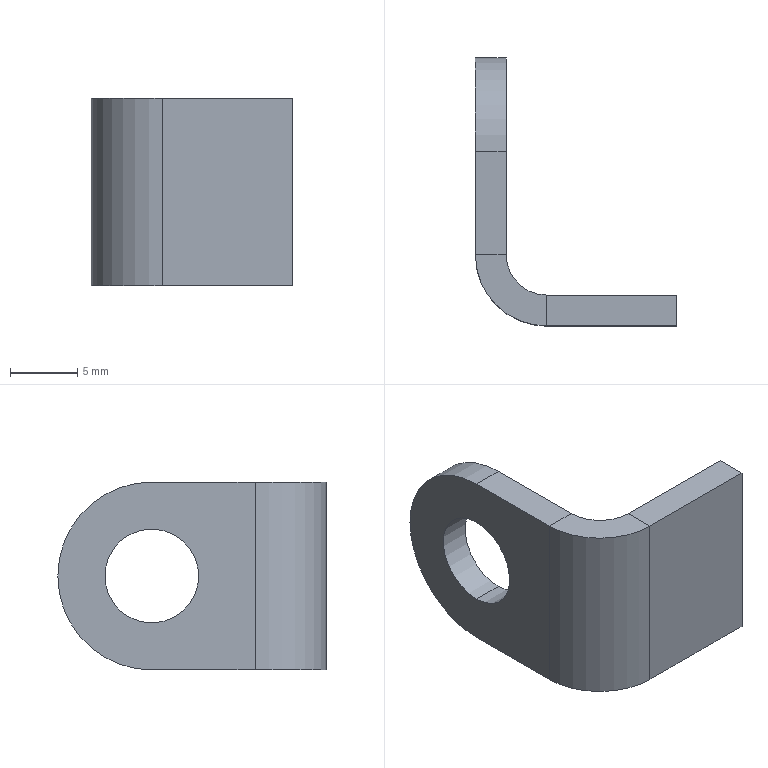Part | SolidWorks | features Fillet 1, FlatPattern 1, ICE 1, SMBaseFlange 1, SheetMetal 1 | 1 solid | 17 faces | box 15 x 20 x 14 mm | volume 858.7 mm3 | plane 11 | cylinder 6 | commonest cylinder face diameters 7 x2 14 x2 6 x1 10.6 x1
STEP:
#1=CARTESIAN_POINT('',(0.,13.,3.5));
#2=VERTEX_POINT('',#1);
#3=CARTESIAN_POINT('',(0.,13.,-3.5));
#4=VERTEX_POINT('',#3);
#5=CARTESIAN_POINT('',(0.,13.,0.));
#6=DIRECTION('',(1.,0.,0.));
#7=DIRECTION('',(0.,0.,-1.));
#8=AXIS2_PLACEMENT_3D('',#5,#6,#7);
#9=CIRCLE('',#8,3.5);
#10=EDGE_CURVE('',#2,#4,#9,.T.);
#11=ORIENTED_EDGE('',*,*,#10,.F.);
#12=CARTESIAN_POINT('',(2.3,13.,3.5));
#13=VERTEX_POINT('',#12);
#14=CARTESIAN_POINT('',(0.,13.,3.5));
#15=DIRECTION('',(1.,0.,0.));
#16=VECTOR('',#15,1000.);
#17=LINE('',#14,#16);
#18=EDGE_CURVE('',#2,#13,#17,.T.);
#19=ORIENTED_EDGE('',*,*,#18,.T.);
#20=CARTESIAN_POINT('',(2.3,13.,-3.5));
#21=VERTEX_POINT('',#20);
#22=CARTESIAN_POINT('',(2.3,13.,0.));
#23=DIRECTION('',(1.,0.,0.));
#24=DIRECTION('',(0.,0.,-1.));
#25=AXIS2_PLACEMENT_3D('',#22,#23,#24);
#26=CIRCLE('',#25,3.5);
#27=EDGE_CURVE('',#13,#21,#26,.T.);
#28=ORIENTED_EDGE('',*,*,#27,.T.);
#29=CARTESIAN_POINT('',(0.,13.,-3.5));
#30=DIRECTION('',(1.,0.,0.));
#31=VECTOR('',#30,1000.);
#32=LINE('',#29,#31);
#33=EDGE_CURVE('',#4,#21,#32,.T.);
#34=ORIENTED_EDGE('',*,*,#33,.F.);
#35=EDGE_LOOP('',(#11,#19,#28,#34));
#36=FACE_OUTER_BOUND('',#35,.T.);
#37=CARTESIAN_POINT('',(0.,13.,0.));
#38=DIRECTION('',(1.,0.,0.));
#39=DIRECTION('',(0.,0.,-1.));
#40=AXIS2_PLACEMENT_3D('',#37,#38,#39);
#41=CYLINDRICAL_SURFACE('',#40,3.5);
#42=ADVANCED_FACE('',(#36),#41,.F.);
#43=CARTESIAN_POINT('',(0.,5.3,7.));
#44=VERTEX_POINT('',#43);
#45=CARTESIAN_POINT('',(2.3,5.3,7.));
#46=VERTEX_POINT('',#45);
#47=CARTESIAN_POINT('',(0.,5.3,7.));
#48=DIRECTION('',(1.,0.,0.));
#49=VECTOR('',#48,1000.);
#50=LINE('',#47,#49);
#51=EDGE_CURVE('',#44,#46,#50,.T.);
#52=ORIENTED_EDGE('',*,*,#51,.F.);
#53=CARTESIAN_POINT('',(5.3,0.,7.));
#54=VERTEX_POINT('',#53);
#55=CARTESIAN_POINT('',(5.3,5.3,7.));
#56=DIRECTION('',(0.,0.,-1.));
#57=DIRECTION('',(1.,0.,0.));
#58=AXIS2_PLACEMENT_3D('',#55,#56,#57);
#59=CIRCLE('',#58,5.3);
#60=EDGE_CURVE('',#54,#44,#59,.T.);
#61=ORIENTED_EDGE('',*,*,#60,.F.);
#62=CARTESIAN_POINT('',(5.3,2.3,7.));
#63=VERTEX_POINT('',#62);
#64=CARTESIAN_POINT('',(5.3,2.3,7.));
#65=DIRECTION('',(0.,-1.,0.));
#66=VECTOR('',#65,1000.);
#67=LINE('',#64,#66);
#68=EDGE_CURVE('',#63,#54,#67,.T.);
#69=ORIENTED_EDGE('',*,*,#68,.F.);
#70=CARTESIAN_POINT('',(5.3,5.3,7.));
#71=DIRECTION('',(0.,0.,-1.));
#72=DIRECTION('',(1.,0.,0.));
#73=AXIS2_PLACEMENT_3D('',#70,#71,#72);
#74=CIRCLE('',#73,3.);
#75=EDGE_CURVE('',#63,#46,#74,.T.);
#76=ORIENTED_EDGE('',*,*,#75,.T.);
#77=EDGE_LOOP('',(#52,#61,#69,#76));
#78=FACE_OUTER_BOUND('',#77,.T.);
#79=CARTESIAN_POINT('',(0.,5.3,7.));
#80=DIRECTION('',(0.,0.,1.));
#81=DIRECTION('',(1.,0.,0.));
#82=AXIS2_PLACEMENT_3D('',#79,#80,#81);
#83=PLANE('',#82);
#84=ADVANCED_FACE('',(#78),#83,.T.);
#85=CARTESIAN_POINT('',(2.3,13.,7.));
#86=VERTEX_POINT('',#85);
#87=CARTESIAN_POINT('',(2.3,0.,7.));
#88=DIRECTION('',(0.,1.,0.));
#89=VECTOR('',#88,1000.);
#90=LINE('',#87,#89);
#91=EDGE_CURVE('',#46,#86,#90,.T.);
#92=ORIENTED_EDGE('',*,*,#91,.T.);
#93=CARTESIAN_POINT('',(0.,13.,7.));
#94=VERTEX_POINT('',#93);
#95=CARTESIAN_POINT('',(5.3,13.,7.));
#96=DIRECTION('',(-1.,0.,0.));
#97=VECTOR('',#96,1000.);
#98=LINE('',#95,#97);
#99=EDGE_CURVE('',#86,#94,#98,.T.);
#100=ORIENTED_EDGE('',*,*,#99,.T.);
#101=CARTESIAN_POINT('',(0.,0.,7.));
#102=DIRECTION('',(0.,1.,0.));
#103=VECTOR('',#102,1000.);
#104=LINE('',#101,#103);
#105=EDGE_CURVE('',#44,#94,#104,.T.);
#106=ORIENTED_EDGE('',*,*,#105,.F.);
#107=ORIENTED_EDGE('',*,*,#51,.T.);
#108=EDGE_LOOP('',(#92,#100,#106,#107));
#109=FACE_OUTER_BOUND('',#108,.T.);
#110=CARTESIAN_POINT('',(5.3,2.3,7.));
#111=DIRECTION('',(0.,0.,1.));
#112=DIRECTION('',(1.,0.,0.));
#113=AXIS2_PLACEMENT_3D('',#110,#111,#112);
#114=PLANE('',#113);
#115=ADVANCED_FACE('',(#109),#114,.T.);
#116=CARTESIAN_POINT('',(5.3,0.,-7.));
#117=VERTEX_POINT('',#116);
#118=CARTESIAN_POINT('',(5.3,2.3,-7.));
#119=VERTEX_POINT('',#118);
#120=CARTESIAN_POINT('',(5.3,0.,-7.));
#121=DIRECTION('',(0.,1.,0.));
#122=VECTOR('',#121,1000.);
#123=LINE('',#120,#122);
#124=EDGE_CURVE('',#117,#119,#123,.T.);
#125=ORIENTED_EDGE('',*,*,#124,.F.);
#126=CARTESIAN_POINT('',(0.,5.3,-7.));
#127=VERTEX_POINT('',#126);
#128=CARTESIAN_POINT('',(5.3,5.3,-7.));
#129=DIRECTION('',(0.,0.,-1.));
#130=DIRECTION('',(1.,0.,0.));
#131=AXIS2_PLACEMENT_3D('',#128,#129,#130);
#132=CIRCLE('',#131,5.3);
#133=EDGE_CURVE('',#117,#127,#132,.T.);
#134=ORIENTED_EDGE('',*,*,#133,.T.);
#135=CARTESIAN_POINT('',(2.3,5.3,-7.));
#136=VERTEX_POINT('',#135);
#137=CARTESIAN_POINT('',(2.3,5.3,-7.));
#138=DIRECTION('',(-1.,0.,0.));
#139=VECTOR('',#138,1000.);
#140=LINE('',#137,#139);
#141=EDGE_CURVE('',#136,#127,#140,.T.);
#142=ORIENTED_EDGE('',*,*,#141,.F.);
#143=CARTESIAN_POINT('',(5.3,5.3,-7.));
#144=DIRECTION('',(0.,0.,-1.));
#145=DIRECTION('',(1.,0.,0.));
#146=AXIS2_PLACEMENT_3D('',#143,#144,#145);
#147=CIRCLE('',#146,3.);
#148=EDGE_CURVE('',#119,#136,#147,.T.);
#149=ORIENTED_EDGE('',*,*,#148,.F.);
#150=EDGE_LOOP('',(#125,#134,#142,#149));
#151=FACE_OUTER_BOUND('',#150,.T.);
#152=CARTESIAN_POINT('',(5.3,0.,-7.));
#153=DIRECTION('',(0.,0.,-1.));
#154=DIRECTION('',(-1.,0.,0.));
#155=AXIS2_PLACEMENT_3D('',#152,#153,#154);
#156=PLANE('',#155);
#157=ADVANCED_FACE('',(#151),#156,.T.);
#158=CARTESIAN_POINT('',(15.,0.,-7.));
#159=VERTEX_POINT('',#158);
#160=CARTESIAN_POINT('',(0.,0.,-7.));
#161=DIRECTION('',(-1.,0.,0.));
#162=VECTOR('',#161,1000.);
#163=LINE('',#160,#162);
#164=EDGE_CURVE('',#159,#117,#163,.T.);
#165=ORIENTED_EDGE('',*,*,#164,.T.);
#166=ORIENTED_EDGE('',*,*,#124,.T.);
#167=CARTESIAN_POINT('',(15.,2.3,-7.));
#168=VERTEX_POINT('',#167);
#169=CARTESIAN_POINT('',(0.,2.3,-7.));
#170=DIRECTION('',(-1.,0.,0.));
#171=VECTOR('',#170,1000.);
#172=LINE('',#169,#171);
#173=EDGE_CURVE('',#168,#119,#172,.T.);
#174=ORIENTED_EDGE('',*,*,#173,.F.);
#175=CARTESIAN_POINT('',(15.,2.3,-7.));
#176=DIRECTION('',(0.,-1.,0.));
#177=VECTOR('',#176,1000.);
#178=LINE('',#175,#177);
#179=EDGE_CURVE('',#168,#159,#178,.T.);
#180=ORIENTED_EDGE('',*,*,#179,.T.);
#181=EDGE_LOOP('',(#165,#166,#174,#180));
#182=FACE_OUTER_BOUND('',#181,.T.);
#183=CARTESIAN_POINT('',(2.3,5.3,-7.));
#184=DIRECTION('',(0.,0.,-1.));
#185=DIRECTION('',(-1.,0.,0.));
#186=AXIS2_PLACEMENT_3D('',#183,#184,#185);
#187=PLANE('',#186);
#188=ADVANCED_FACE('',(#182),#187,.T.);
#189=CARTESIAN_POINT('',(2.3,13.,0.));
#190=DIRECTION('',(1.,0.,0.));
#191=DIRECTION('',(0.,0.,-1.));
#192=AXIS2_PLACEMENT_3D('',#189,#190,#191);
#193=CIRCLE('',#192,3.5);
#194=EDGE_CURVE('',#21,#13,#193,.T.);
#195=ORIENTED_EDGE('',*,*,#194,.F.);
#196=ORIENTED_EDGE('',*,*,#27,.F.);
#197=EDGE_LOOP('',(#195,#196));
#198=FACE_BOUND('',#197,.T.);
#199=CARTESIAN_POINT('',(2.3,13.,-7.));
#200=VERTEX_POINT('',#199);
#201=CARTESIAN_POINT('',(2.3,0.,-7.));
#202=DIRECTION('',(0.,1.,0.));
#203=VECTOR('',#202,1000.);
#204=LINE('',#201,#203);
#205=EDGE_CURVE('',#136,#200,#204,.T.);
#206=ORIENTED_EDGE('',*,*,#205,.T.);
#207=CARTESIAN_POINT('',(2.3,20.,0.));
#208=VERTEX_POINT('',#207);
#209=CARTESIAN_POINT('',(2.3,13.,0.));
#210=DIRECTION('',(1.,0.,0.));
#211=DIRECTION('',(0.,0.,1.));
#212=AXIS2_PLACEMENT_3D('',#209,#210,#211);
#213=CIRCLE('',#212,7.);
#214=EDGE_CURVE('',#200,#208,#213,.T.);
#215=ORIENTED_EDGE('',*,*,#214,.T.);
#216=CARTESIAN_POINT('',(2.3,13.,0.));
#217=DIRECTION('',(1.,0.,0.));
#218=DIRECTION('',(0.,0.,1.));
#219=AXIS2_PLACEMENT_3D('',#216,#217,#218);
#220=CIRCLE('',#219,7.);
#221=EDGE_CURVE('',#208,#86,#220,.T.);
#222=ORIENTED_EDGE('',*,*,#221,.T.);
#223=ORIENTED_EDGE('',*,*,#91,.F.);
#224=CARTESIAN_POINT('',(2.3,5.3,7.));
#225=DIRECTION('',(0.,0.,-1.));
#226=VECTOR('',#225,1000.);
#227=LINE('',#224,#226);
#228=EDGE_CURVE('',#46,#136,#227,.T.);
#229=ORIENTED_EDGE('',*,*,#228,.T.);
#230=EDGE_LOOP('',(#206,#215,#222,#223,#229));
#231=FACE_OUTER_BOUND('',#230,.T.);
#232=CARTESIAN_POINT('',(2.3,0.,7.));
#233=DIRECTION('',(-1.,0.,0.));
#234=DIRECTION('',(0.,0.,1.));
#235=AXIS2_PLACEMENT_3D('',#232,#233,#234);
#236=PLANE('',#235);
#237=ADVANCED_FACE('',(#198,#231),#236,.F.);
#238=CARTESIAN_POINT('',(0.,13.,0.));
#239=DIRECTION('',(1.,0.,0.));
#240=DIRECTION('',(0.,0.,-1.));
#241=AXIS2_PLACEMENT_3D('',#238,#239,#240);
#242=CIRCLE('',#241,3.5);
#243=EDGE_CURVE('',#4,#2,#242,.T.);
#244=ORIENTED_EDGE('',*,*,#243,.T.);
#245=ORIENTED_EDGE('',*,*,#10,.T.);
#246=EDGE_LOOP('',(#244,#245));
#247=FACE_BOUND('',#246,.T.);
#248=CARTESIAN_POINT('',(0.,20.,0.));
#249=VERTEX_POINT('',#248);
#250=CARTESIAN_POINT('',(0.,13.,0.));
#251=DIRECTION('',(-1.,0.,0.));
#252=DIRECTION('',(0.,0.,1.));
#253=AXIS2_PLACEMENT_3D('',#250,#251,#252);
#254=CIRCLE('',#253,7.);
#255=EDGE_CURVE('',#94,#249,#254,.T.);
#256=ORIENTED_EDGE('',*,*,#255,.T.);
#257=CARTESIAN_POINT('',(0.,13.,-7.));
#258=VERTEX_POINT('',#257);
#259=CARTESIAN_POINT('',(0.,13.,0.));
#260=DIRECTION('',(-1.,0.,0.));
#261=DIRECTION('',(0.,0.,1.));
#262=AXIS2_PLACEMENT_3D('',#259,#260,#261);
#263=CIRCLE('',#262,7.);
#264=EDGE_CURVE('',#249,#258,#263,.T.);
#265=ORIENTED_EDGE('',*,*,#264,.T.);
#266=CARTESIAN_POINT('',(0.,0.,-7.));
#267=DIRECTION('',(0.,1.,0.));
#268=VECTOR('',#267,1000.);
#269=LINE('',#266,#268);
#270=EDGE_CURVE('',#127,#258,#269,.T.);
#271=ORIENTED_EDGE('',*,*,#270,.F.);
#272=CARTESIAN_POINT('',(0.,5.3,7.));
#273=DIRECTION('',(0.,0.,-1.));
#274=VECTOR('',#273,1000.);
#275=LINE('',#272,#274);
#276=EDGE_CURVE('',#44,#127,#275,.T.);
#277=ORIENTED_EDGE('',*,*,#276,.F.);
#278=ORIENTED_EDGE('',*,*,#105,.T.);
#279=EDGE_LOOP('',(#256,#265,#271,#277,#278));
#280=FACE_OUTER_BOUND('',#279,.T.);
#281=CARTESIAN_POINT('',(0.,0.,7.));
#282=DIRECTION('',(-1.,0.,0.));
#283=DIRECTION('',(0.,0.,1.));
#284=AXIS2_PLACEMENT_3D('',#281,#282,#283);
#285=PLANE('',#284);
#286=ADVANCED_FACE('',(#247,#280),#285,.T.);
#287=ORIENTED_EDGE('',*,*,#133,.F.);
#288=CARTESIAN_POINT('',(5.3,0.,7.));
#289=DIRECTION('',(0.,0.,-1.));
#290=VECTOR('',#289,1000.);
#291=LINE('',#288,#290);
#292=EDGE_CURVE('',#54,#117,#291,.T.);
#293=ORIENTED_EDGE('',*,*,#292,.F.);
#294=ORIENTED_EDGE('',*,*,#60,.T.);
#295=ORIENTED_EDGE('',*,*,#276,.T.);
#296=EDGE_LOOP('',(#287,#293,#294,#295));
#297=FACE_OUTER_BOUND('',#296,.T.);
#298=CARTESIAN_POINT('',(5.3,5.3,7.));
#299=DIRECTION('',(0.,0.,-1.));
#300=DIRECTION('',(-1.,0.,0.));
#301=AXIS2_PLACEMENT_3D('',#298,#299,#300);
#302=CYLINDRICAL_SURFACE('',#301,5.3);
#303=ADVANCED_FACE('',(#297),#302,.T.);
#304=ORIENTED_EDGE('',*,*,#164,.F.);
#305=CARTESIAN_POINT('',(15.,0.,7.));
#306=VERTEX_POINT('',#305);
#307=CARTESIAN_POINT('',(15.,0.,7.));
#308=DIRECTION('',(0.,0.,-1.));
#309=VECTOR('',#308,1000.);
#310=LINE('',#307,#309);
#311=EDGE_CURVE('',#306,#159,#310,.T.);
#312=ORIENTED_EDGE('',*,*,#311,.F.);
#313=CARTESIAN_POINT('',(0.,0.,7.));
#314=DIRECTION('',(-1.,0.,0.));
#315=VECTOR('',#314,1000.);
#316=LINE('',#313,#315);
#317=EDGE_CURVE('',#306,#54,#316,.T.);
#318=ORIENTED_EDGE('',*,*,#317,.T.);
#319=ORIENTED_EDGE('',*,*,#292,.T.);
#320=EDGE_LOOP('',(#304,#312,#318,#319));
#321=FACE_OUTER_BOUND('',#320,.T.);
#322=CARTESIAN_POINT('',(0.,0.,7.));
#323=DIRECTION('',(0.,-1.,0.));
#324=DIRECTION('',(0.,0.,-1.));
#325=AXIS2_PLACEMENT_3D('',#322,#323,#324);
#326=PLANE('',#325);
#327=ADVANCED_FACE('',(#321),#326,.T.);
#328=ORIENTED_EDGE('',*,*,#179,.F.);
#329=CARTESIAN_POINT('',(15.,2.3,7.));
#330=VERTEX_POINT('',#329);
#331=CARTESIAN_POINT('',(15.,2.3,7.));
#332=DIRECTION('',(0.,0.,-1.));
#333=VECTOR('',#332,1000.);
#334=LINE('',#331,#333);
#335=EDGE_CURVE('',#330,#168,#334,.T.);
#336=ORIENTED_EDGE('',*,*,#335,.F.);
#337=CARTESIAN_POINT('',(15.,2.3,7.));
#338=DIRECTION('',(0.,-1.,0.));
#339=VECTOR('',#338,1000.);
#340=LINE('',#337,#339);
#341=EDGE_CURVE('',#330,#306,#340,.T.);
#342=ORIENTED_EDGE('',*,*,#341,.T.);
#343=ORIENTED_EDGE('',*,*,#311,.T.);
#344=EDGE_LOOP('',(#328,#336,#342,#343));
#345=FACE_OUTER_BOUND('',#344,.T.);
#346=CARTESIAN_POINT('',(15.,2.3,7.));
#347=DIRECTION('',(1.,0.,0.));
#348=DIRECTION('',(0.,0.,-1.));
#349=AXIS2_PLACEMENT_3D('',#346,#347,#348);
#350=PLANE('',#349);
#351=ADVANCED_FACE('',(#345),#350,.T.);
#352=ORIENTED_EDGE('',*,*,#173,.T.);
#353=CARTESIAN_POINT('',(5.3,2.3,7.));
#354=DIRECTION('',(0.,0.,-1.));
#355=VECTOR('',#354,1000.);
#356=LINE('',#353,#355);
#357=EDGE_CURVE('',#63,#119,#356,.T.);
#358=ORIENTED_EDGE('',*,*,#357,.F.);
#359=CARTESIAN_POINT('',(0.,2.3,7.));
#360=DIRECTION('',(-1.,0.,0.));
#361=VECTOR('',#360,1000.);
#362=LINE('',#359,#361);
#363=EDGE_CURVE('',#330,#63,#362,.T.);
#364=ORIENTED_EDGE('',*,*,#363,.F.);
#365=ORIENTED_EDGE('',*,*,#335,.T.);
#366=EDGE_LOOP('',(#352,#358,#364,#365));
#367=FACE_OUTER_BOUND('',#366,.T.);
#368=CARTESIAN_POINT('',(0.,2.3,7.));
#369=DIRECTION('',(0.,-1.,0.));
#370=DIRECTION('',(0.,0.,-1.));
#371=AXIS2_PLACEMENT_3D('',#368,#369,#370);
#372=PLANE('',#371);
#373=ADVANCED_FACE('',(#367),#372,.F.);
#374=ORIENTED_EDGE('',*,*,#148,.T.);
#375=ORIENTED_EDGE('',*,*,#228,.F.);
#376=ORIENTED_EDGE('',*,*,#75,.F.);
#377=ORIENTED_EDGE('',*,*,#357,.T.);
#378=EDGE_LOOP('',(#374,#375,#376,#377));
#379=FACE_OUTER_BOUND('',#378,.T.);
#380=CARTESIAN_POINT('',(5.3,5.3,7.));
#381=DIRECTION('',(0.,0.,-1.));
#382=DIRECTION('',(-1.,0.,0.));
#383=AXIS2_PLACEMENT_3D('',#380,#381,#382);
#384=CYLINDRICAL_SURFACE('',#383,3.);
#385=ADVANCED_FACE('',(#379),#384,.F.);
#386=ORIENTED_EDGE('',*,*,#363,.T.);
#387=ORIENTED_EDGE('',*,*,#68,.T.);
#388=ORIENTED_EDGE('',*,*,#317,.F.);
#389=ORIENTED_EDGE('',*,*,#341,.F.);
#390=EDGE_LOOP('',(#386,#387,#388,#389));
#391=FACE_OUTER_BOUND('',#390,.T.);
#392=CARTESIAN_POINT('',(5.3,5.3,7.));
#393=DIRECTION('',(0.,0.,1.));
#394=DIRECTION('',(1.,0.,0.));
#395=AXIS2_PLACEMENT_3D('',#392,#393,#394);
#396=PLANE('',#395);
#397=ADVANCED_FACE('',(#391),#396,.T.);
#398=ORIENTED_EDGE('',*,*,#270,.T.);
#399=CARTESIAN_POINT('',(2.3,13.,-7.));
#400=DIRECTION('',(1.,0.,0.));
#401=VECTOR('',#400,1000.);
#402=LINE('',#399,#401);
#403=EDGE_CURVE('',#258,#200,#402,.T.);
#404=ORIENTED_EDGE('',*,*,#403,.T.);
#405=ORIENTED_EDGE('',*,*,#205,.F.);
#406=ORIENTED_EDGE('',*,*,#141,.T.);
#407=EDGE_LOOP('',(#398,#404,#405,#406));
#408=FACE_OUTER_BOUND('',#407,.T.);
#409=CARTESIAN_POINT('',(5.3,5.3,-7.));
#410=DIRECTION('',(0.,0.,1.));
#411=DIRECTION('',(1.,0.,0.));
#412=AXIS2_PLACEMENT_3D('',#409,#410,#411);
#413=PLANE('',#412);
#414=ADVANCED_FACE('',(#408),#413,.F.);
#415=ORIENTED_EDGE('',*,*,#18,.F.);
#416=ORIENTED_EDGE('',*,*,#243,.F.);
#417=ORIENTED_EDGE('',*,*,#33,.T.);
#418=ORIENTED_EDGE('',*,*,#194,.T.);
#419=EDGE_LOOP('',(#415,#416,#417,#418));
#420=FACE_OUTER_BOUND('',#419,.T.);
#421=CARTESIAN_POINT('',(0.,13.,0.));
#422=DIRECTION('',(1.,0.,0.));
#423=DIRECTION('',(0.,0.,-1.));
#424=AXIS2_PLACEMENT_3D('',#421,#422,#423);
#425=CYLINDRICAL_SURFACE('',#424,3.5);
#426=ADVANCED_FACE('',(#420),#425,.F.);
#427=CARTESIAN_POINT('',(0.,20.,0.));
#428=DIRECTION('',(1.,0.,0.));
#429=VECTOR('',#428,1000.);
#430=LINE('',#427,#429);
#431=EDGE_CURVE('',#249,#208,#430,.T.);
#432=ORIENTED_EDGE('',*,*,#431,.F.);
#433=ORIENTED_EDGE('',*,*,#255,.F.);
#434=ORIENTED_EDGE('',*,*,#99,.F.);
#435=ORIENTED_EDGE('',*,*,#221,.F.);
#436=EDGE_LOOP('',(#432,#433,#434,#435));
#437=FACE_OUTER_BOUND('',#436,.T.);
#438=CARTESIAN_POINT('',(0.,13.,0.));
#439=DIRECTION('',(1.,0.,0.));
#440=DIRECTION('',(0.,0.,-1.));
#441=AXIS2_PLACEMENT_3D('',#438,#439,#440);
#442=CYLINDRICAL_SURFACE('',#441,7.);
#443=ADVANCED_FACE('',(#437),#442,.T.);
#444=ORIENTED_EDGE('',*,*,#264,.F.);
#445=ORIENTED_EDGE('',*,*,#431,.T.);
#446=ORIENTED_EDGE('',*,*,#214,.F.);
#447=ORIENTED_EDGE('',*,*,#403,.F.);
#448=EDGE_LOOP('',(#444,#445,#446,#447));
#449=FACE_OUTER_BOUND('',#448,.T.);
#450=CARTESIAN_POINT('',(5.3,13.,0.));
#451=DIRECTION('',(-1.,0.,0.));
#452=DIRECTION('',(0.,0.,1.));
#453=AXIS2_PLACEMENT_3D('',#450,#451,#452);
#454=CYLINDRICAL_SURFACE('',#453,7.);
#455=ADVANCED_FACE('',(#449),#454,.T.);
#456=CLOSED_SHELL('',(#42,#84,#115,#157,#188,#237,#286,#303,#327,#351,#373,#385,#397,#414,#426,#443,#455));
#457=MANIFOLD_SOLID_BREP('',#456);
#458=CARTESIAN_POINT('',(0.,0.,0.));
#459=DIRECTION('',(0.,0.,1.));
#460=DIRECTION('',(1.,0.,0.));
#461=AXIS2_PLACEMENT_3D('',#458,#459,#460);
#462=(LENGTH_UNIT()NAMED_UNIT(*)SI_UNIT(.MILLI.,.METRE.));
#463=UNCERTAINTY_MEASURE_WITH_UNIT(LENGTH_MEASURE(0.00001),#462,'','');
#464=(NAMED_UNIT(*)PLANE_ANGLE_UNIT()SI_UNIT($,.RADIAN.));
#465=(NAMED_UNIT(*)SI_UNIT($,.STERADIAN.)SOLID_ANGLE_UNIT());
#466=(GEOMETRIC_REPRESENTATION_CONTEXT(3)GLOBAL_UNCERTAINTY_ASSIGNED_CONTEXT((#463))GLOBAL_UNIT_ASSIGNED_CONTEXT((#462,#464,#465))REPRESENTATION_CONTEXT('',''));
#467=ADVANCED_BREP_SHAPE_REPRESENTATION('',(#457,#461),#466);